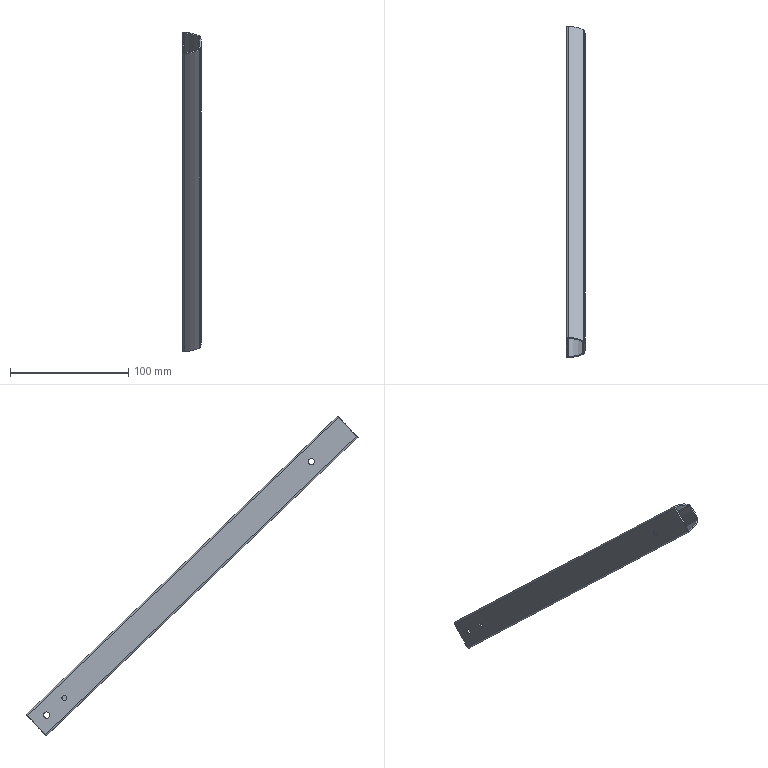Part | SolidWorks | features BaseBody 1 | 1 solid | 30 faces | box 16 x 280.261 x 269.738 mm | volume 29192 mm3 | cylinder 26 | plane 4 | commonest cylinder face diameters 5.2 x8 0.6 x3 3 x3 3.6 x2 4.2 x2 6 x2
STEP:
#1=CARTESIAN_POINT('',(173.2,660.373,82.941));
#2=VERTEX_POINT('',#1);
#3=CARTESIAN_POINT('',(173.2,660.373,87.141));
#4=VERTEX_POINT('',#3);
#5=CARTESIAN_POINT('',(173.2,660.373,85.041));
#6=DIRECTION('',(-1.,0.,0.));
#7=DIRECTION('',(0.,0.,1.));
#8=AXIS2_PLACEMENT_3D('',#5,#6,#7);
#9=CIRCLE('',#8,2.1);
#10=EDGE_CURVE('',#2,#4,#9,.T.);
#11=ORIENTED_EDGE('',*,*,#10,.F.);
#12=CARTESIAN_POINT('',(172.,660.373,82.941));
#13=VERTEX_POINT('',#12);
#14=CARTESIAN_POINT('',(182.,660.373,82.941));
#15=DIRECTION('',(-1.,0.,0.));
#16=VECTOR('',#15,1000.);
#17=LINE('',#14,#16);
#18=EDGE_CURVE('',#2,#13,#17,.T.);
#19=ORIENTED_EDGE('',*,*,#18,.T.);
#20=CARTESIAN_POINT('',(172.,660.373,87.141));
#21=VERTEX_POINT('',#20);
#22=CARTESIAN_POINT('',(172.,660.373,85.041));
#23=DIRECTION('',(1.,0.,0.));
#24=DIRECTION('',(0.,0.,1.));
#25=AXIS2_PLACEMENT_3D('',#22,#23,#24);
#26=CIRCLE('',#25,2.1);
#27=EDGE_CURVE('',#21,#13,#26,.T.);
#28=ORIENTED_EDGE('',*,*,#27,.F.);
#29=CARTESIAN_POINT('',(182.,660.373,87.141));
#30=DIRECTION('',(-1.,0.,0.));
#31=VECTOR('',#30,1000.);
#32=LINE('',#29,#31);
#33=EDGE_CURVE('',#4,#21,#32,.T.);
#34=ORIENTED_EDGE('',*,*,#33,.F.);
#35=EDGE_LOOP('',(#11,#19,#28,#34));
#36=FACE_OUTER_BOUND('',#35,.T.);
#37=CARTESIAN_POINT('',(182.,660.373,85.041));
#38=DIRECTION('',(-1.,0.,0.));
#39=DIRECTION('',(0.,0.,1.));
#40=AXIS2_PLACEMENT_3D('',#37,#38,#39);
#41=CYLINDRICAL_SURFACE('',#40,2.1);
#42=ADVANCED_FACE('',(#36),#41,.F.);
#43=CARTESIAN_POINT('',(172.,675.31,73.346));
#44=VERTEX_POINT('',#43);
#45=CARTESIAN_POINT('',(172.,675.31,68.146));
#46=VERTEX_POINT('',#45);
#47=CARTESIAN_POINT('',(172.,675.31,70.746));
#48=DIRECTION('',(1.,0.,0.));
#49=DIRECTION('',(0.,0.,-1.));
#50=AXIS2_PLACEMENT_3D('',#47,#48,#49);
#51=CIRCLE('',#50,2.6);
#52=EDGE_CURVE('',#44,#46,#51,.T.);
#53=ORIENTED_EDGE('',*,*,#52,.F.);
#54=CARTESIAN_POINT('',(173.2,675.31,73.346));
#55=VERTEX_POINT('',#54);
#56=CARTESIAN_POINT('',(133.,675.31,73.346));
#57=DIRECTION('',(1.,0.,0.));
#58=VECTOR('',#57,1000.);
#59=LINE('',#56,#58);
#60=EDGE_CURVE('',#44,#55,#59,.T.);
#61=ORIENTED_EDGE('',*,*,#60,.T.);
#62=CARTESIAN_POINT('',(173.2,675.31,68.146));
#63=VERTEX_POINT('',#62);
#64=CARTESIAN_POINT('',(173.2,675.31,70.746));
#65=DIRECTION('',(-1.,0.,0.));
#66=DIRECTION('',(0.,0.,-1.));
#67=AXIS2_PLACEMENT_3D('',#64,#65,#66);
#68=CIRCLE('',#67,2.6);
#69=EDGE_CURVE('',#63,#55,#68,.T.);
#70=ORIENTED_EDGE('',*,*,#69,.F.);
#71=CARTESIAN_POINT('',(133.,675.31,68.146));
#72=DIRECTION('',(1.,0.,0.));
#73=VECTOR('',#72,1000.);
#74=LINE('',#71,#73);
#75=EDGE_CURVE('',#46,#63,#74,.T.);
#76=ORIENTED_EDGE('',*,*,#75,.F.);
#77=EDGE_LOOP('',(#53,#61,#70,#76));
#78=FACE_OUTER_BOUND('',#77,.T.);
#79=CARTESIAN_POINT('',(133.,675.31,70.746));
#80=DIRECTION('',(1.,0.,0.));
#81=DIRECTION('',(0.,0.,-1.));
#82=AXIS2_PLACEMENT_3D('',#79,#80,#81);
#83=CYLINDRICAL_SURFACE('',#82,2.6);
#84=ADVANCED_FACE('',(#78),#83,.F.);
#85=CARTESIAN_POINT('',(172.,428.723,321.908));
#86=VERTEX_POINT('',#85);
#87=CARTESIAN_POINT('',(173.5,429.76,322.992));
#88=VERTEX_POINT('',#87);
#89=CARTESIAN_POINT('',(173.5,428.723,321.908));
#90=DIRECTION('',(0.,0.7224,-0.6914));
#91=DIRECTION('',(0.,0.6914,0.7224));
#92=AXIS2_PLACEMENT_3D('',#89,#90,#91);
#93=CIRCLE('',#92,1.5);
#94=EDGE_CURVE('',#86,#88,#93,.T.);
#95=ORIENTED_EDGE('',*,*,#94,.T.);
#96=CARTESIAN_POINT('',(173.5,692.797,71.25));
#97=VERTEX_POINT('',#96);
#98=CARTESIAN_POINT('',(173.5,-6.027,740.064));
#99=DIRECTION('',(0.,0.7224,-0.6914));
#100=VECTOR('',#99,1000.);
#101=LINE('',#98,#100);
#102=EDGE_CURVE('',#88,#97,#101,.T.);
#103=ORIENTED_EDGE('',*,*,#102,.T.);
#104=CARTESIAN_POINT('',(172.,691.76,70.167));
#105=VERTEX_POINT('',#104);
#106=CARTESIAN_POINT('',(173.5,691.76,70.167));
#107=DIRECTION('',(0.,0.7224,-0.6914));
#108=DIRECTION('',(0.,0.6914,0.7224));
#109=AXIS2_PLACEMENT_3D('',#106,#107,#108);
#110=CIRCLE('',#109,1.5);
#111=EDGE_CURVE('',#105,#97,#110,.T.);
#112=ORIENTED_EDGE('',*,*,#111,.F.);
#113=CARTESIAN_POINT('',(172.,428.723,321.908));
#114=DIRECTION('',(0.,0.7224,-0.6914));
#115=VECTOR('',#114,1000.);
#116=LINE('',#113,#115);
#117=EDGE_CURVE('',#86,#105,#116,.T.);
#118=ORIENTED_EDGE('',*,*,#117,.F.);
#119=EDGE_LOOP('',(#95,#103,#112,#118));
#120=FACE_OUTER_BOUND('',#119,.T.);
#121=CARTESIAN_POINT('',(173.5,-7.064,738.98));
#122=DIRECTION('',(0.,0.7224,-0.6914));
#123=DIRECTION('',(0.,0.6914,0.7224));
#124=AXIS2_PLACEMENT_3D('',#121,#122,#123);
#125=CYLINDRICAL_SURFACE('',#124,1.5);
#126=ADVANCED_FACE('',(#120),#125,.T.);
#127=CARTESIAN_POINT('',(172.,451.846,287.213));
#128=VERTEX_POINT('',#127);
#129=CARTESIAN_POINT('',(172.,451.846,282.013));
#130=VERTEX_POINT('',#129);
#131=CARTESIAN_POINT('',(172.,451.846,284.613));
#132=DIRECTION('',(1.,0.,0.));
#133=DIRECTION('',(0.,0.,-1.));
#134=AXIS2_PLACEMENT_3D('',#131,#132,#133);
#135=CIRCLE('',#134,2.6);
#136=EDGE_CURVE('',#128,#130,#135,.T.);
#137=ORIENTED_EDGE('',*,*,#136,.F.);
#138=CARTESIAN_POINT('',(173.2,451.846,287.213));
#139=VERTEX_POINT('',#138);
#140=CARTESIAN_POINT('',(-462.,451.846,287.213));
#141=DIRECTION('',(1.,0.,0.));
#142=VECTOR('',#141,1000.);
#143=LINE('',#140,#142);
#144=EDGE_CURVE('',#128,#139,#143,.T.);
#145=ORIENTED_EDGE('',*,*,#144,.T.);
#146=CARTESIAN_POINT('',(173.2,451.846,282.013));
#147=VERTEX_POINT('',#146);
#148=CARTESIAN_POINT('',(173.2,451.846,284.613));
#149=DIRECTION('',(-1.,0.,0.));
#150=DIRECTION('',(0.,0.,-1.));
#151=AXIS2_PLACEMENT_3D('',#148,#149,#150);
#152=CIRCLE('',#151,2.6);
#153=EDGE_CURVE('',#147,#139,#152,.T.);
#154=ORIENTED_EDGE('',*,*,#153,.F.);
#155=CARTESIAN_POINT('',(-462.,451.846,282.013));
#156=DIRECTION('',(1.,0.,0.));
#157=VECTOR('',#156,1000.);
#158=LINE('',#155,#157);
#159=EDGE_CURVE('',#130,#147,#158,.T.);
#160=ORIENTED_EDGE('',*,*,#159,.F.);
#161=EDGE_LOOP('',(#137,#145,#154,#160));
#162=FACE_OUTER_BOUND('',#161,.T.);
#163=CARTESIAN_POINT('',(-462.,451.846,284.613));
#164=DIRECTION('',(1.,0.,0.));
#165=DIRECTION('',(0.,0.,-1.));
#166=AXIS2_PLACEMENT_3D('',#163,#164,#165);
#167=CYLINDRICAL_SURFACE('',#166,2.6);
#168=ADVANCED_FACE('',(#162),#167,.F.);
#169=CARTESIAN_POINT('',(173.5,428.93,322.125));
#170=VERTEX_POINT('',#169);
#171=CARTESIAN_POINT('',(173.519,428.93,322.124));
#172=VERTEX_POINT('',#171);
#173=CARTESIAN_POINT('',(173.5,428.723,321.908));
#174=DIRECTION('',(0.,0.7224,-0.6914));
#175=DIRECTION('',(0.,0.6914,0.7224));
#176=AXIS2_PLACEMENT_3D('',#173,#174,#175);
#177=CIRCLE('',#176,0.3);
#178=EDGE_CURVE('',#170,#172,#177,.T.);
#179=ORIENTED_EDGE('',*,*,#178,.F.);
#180=CARTESIAN_POINT('',(173.5,691.967,70.383));
#181=VERTEX_POINT('',#180);
#182=CARTESIAN_POINT('',(173.5,-6.857,739.197));
#183=DIRECTION('',(0.,0.7224,-0.6914));
#184=VECTOR('',#183,1000.);
#185=LINE('',#182,#184);
#186=EDGE_CURVE('',#170,#181,#185,.T.);
#187=ORIENTED_EDGE('',*,*,#186,.T.);
#188=CARTESIAN_POINT('',(173.519,691.967,70.383));
#189=VERTEX_POINT('',#188);
#190=CARTESIAN_POINT('',(173.5,691.76,70.167));
#191=DIRECTION('',(0.,-0.7224,0.6914));
#192=DIRECTION('',(0.,0.6914,0.7224));
#193=AXIS2_PLACEMENT_3D('',#190,#191,#192);
#194=CIRCLE('',#193,0.3);
#195=EDGE_CURVE('',#189,#181,#194,.T.);
#196=ORIENTED_EDGE('',*,*,#195,.F.);
#197=CARTESIAN_POINT('',(173.519,-6.857,739.196));
#198=DIRECTION('',(0.,-0.7224,0.6914));
#199=VECTOR('',#198,1000.);
#200=LINE('',#197,#199);
#201=EDGE_CURVE('',#189,#172,#200,.T.);
#202=ORIENTED_EDGE('',*,*,#201,.T.);
#203=EDGE_LOOP('',(#179,#187,#196,#202));
#204=FACE_OUTER_BOUND('',#203,.T.);
#205=CARTESIAN_POINT('',(173.5,-7.064,738.98));
#206=DIRECTION('',(0.,0.7224,-0.6914));
#207=DIRECTION('',(0.,0.6914,0.7224));
#208=AXIS2_PLACEMENT_3D('',#205,#206,#207);
#209=CYLINDRICAL_SURFACE('',#208,0.3);
#210=ADVANCED_FACE('',(#204),#209,.F.);
#211=CARTESIAN_POINT('',(186.739,675.31,68.146));
#212=VERTEX_POINT('',#211);
#213=CARTESIAN_POINT('',(186.739,675.31,73.346));
#214=VERTEX_POINT('',#213);
#215=CARTESIAN_POINT('',(186.739,675.31,68.146));
#216=CARTESIAN_POINT('',(186.731,675.138,68.146));
#217=CARTESIAN_POINT('',(186.723,674.969,68.163));
#218=CARTESIAN_POINT('',(186.709,674.637,68.229));
#219=CARTESIAN_POINT('',(186.703,674.472,68.279));
#220=CARTESIAN_POINT('',(186.693,674.157,68.41));
#221=CARTESIAN_POINT('',(186.689,674.008,68.49));
#222=CARTESIAN_POINT('',(186.683,673.725,68.678));
#223=CARTESIAN_POINT('',(186.682,673.591,68.788));
#224=CARTESIAN_POINT('',(186.683,673.351,69.028));
#225=CARTESIAN_POINT('',(186.685,673.244,69.159));
#226=CARTESIAN_POINT('',(186.691,673.053,69.443));
#227=CARTESIAN_POINT('',(186.696,672.973,69.595));
#228=CARTESIAN_POINT('',(186.707,672.843,69.907));
#229=CARTESIAN_POINT('',(186.714,672.793,70.071));
#230=CARTESIAN_POINT('',(186.728,672.726,70.407));
#231=CARTESIAN_POINT('',(186.736,672.71,70.575));
#232=CARTESIAN_POINT('',(186.751,672.71,70.914));
#233=CARTESIAN_POINT('',(186.759,672.726,71.086));
#234=CARTESIAN_POINT('',(186.773,672.793,71.42));
#235=CARTESIAN_POINT('',(186.779,672.842,71.582));
#236=CARTESIAN_POINT('',(186.79,672.972,71.896));
#237=CARTESIAN_POINT('',(186.794,673.053,72.049));
#238=CARTESIAN_POINT('',(186.799,673.241,72.331));
#239=CARTESIAN_POINT('',(186.8,673.349,72.462));
#240=CARTESIAN_POINT('',(186.8,673.591,72.705));
#241=CARTESIAN_POINT('',(186.798,673.723,72.813));
#242=CARTESIAN_POINT('',(186.791,674.004,73.001));
#243=CARTESIAN_POINT('',(186.787,674.156,73.083));
#244=CARTESIAN_POINT('',(186.775,674.471,73.213));
#245=CARTESIAN_POINT('',(186.769,674.633,73.263));
#246=CARTESIAN_POINT('',(186.754,674.966,73.329));
#247=CARTESIAN_POINT('',(186.746,675.138,73.346));
#248=CARTESIAN_POINT('',(186.739,675.31,73.346));
#249=B_SPLINE_CURVE_WITH_KNOTS('',3,(#215,#216,#217,#218,#219,#220,#221,#222,#223,#224,#225,#226,#227,#228,#229,#230,#231,#232,#233,#234,#235,#236,#237,#238,#239,#240,#241,#242,#243,#244,#245,#246,#247,#248),.UNSPECIFIED.,.F.,.F.,(4,2,2,2,2,2,2,2,2,2,2,2,2,2,2,2,4),(0.,0.0005082,0.001016,0.001525,0.002033,0.002541,0.003049,0.003557,0.004066,0.004574,0.005082,0.00559,0.006098,0.006607,0.007115,0.007623,0.008131),.UNSPECIFIED.);
#250=EDGE_CURVE('',#212,#214,#249,.T.);
#251=ORIENTED_EDGE('',*,*,#250,.T.);
#252=CARTESIAN_POINT('',(187.941,675.31,73.346));
#253=VERTEX_POINT('',#252);
#254=CARTESIAN_POINT('',(133.,675.31,73.346));
#255=DIRECTION('',(1.,0.,0.));
#256=VECTOR('',#255,1000.);
#257=LINE('',#254,#256);
#258=EDGE_CURVE('',#214,#253,#257,.T.);
#259=ORIENTED_EDGE('',*,*,#258,.T.);
#260=CARTESIAN_POINT('',(187.941,675.31,68.146));
#261=VERTEX_POINT('',#260);
#262=CARTESIAN_POINT('',(187.941,675.31,68.146));
#263=CARTESIAN_POINT('',(187.934,675.138,68.146));
#264=CARTESIAN_POINT('',(187.926,674.969,68.163));
#265=CARTESIAN_POINT('',(187.913,674.637,68.229));
#266=CARTESIAN_POINT('',(187.907,674.472,68.279));
#267=CARTESIAN_POINT('',(187.897,674.157,68.41));
#268=CARTESIAN_POINT('',(187.893,674.008,68.49));
#269=CARTESIAN_POINT('',(187.888,673.725,68.678));
#270=CARTESIAN_POINT('',(187.887,673.591,68.788));
#271=CARTESIAN_POINT('',(187.887,673.351,69.028));
#272=CARTESIAN_POINT('',(187.889,673.244,69.159));
#273=CARTESIAN_POINT('',(187.896,673.053,69.443));
#274=CARTESIAN_POINT('',(187.9,672.973,69.595));
#275=CARTESIAN_POINT('',(187.911,672.843,69.907));
#276=CARTESIAN_POINT('',(187.917,672.793,70.071));
#277=CARTESIAN_POINT('',(187.931,672.726,70.407));
#278=CARTESIAN_POINT('',(187.939,672.71,70.575));
#279=CARTESIAN_POINT('',(187.953,672.71,70.914));
#280=CARTESIAN_POINT('',(187.961,672.726,71.086));
#281=CARTESIAN_POINT('',(187.974,672.793,71.42));
#282=CARTESIAN_POINT('',(187.98,672.842,71.582));
#283=CARTESIAN_POINT('',(187.99,672.972,71.896));
#284=CARTESIAN_POINT('',(187.994,673.053,72.049));
#285=CARTESIAN_POINT('',(187.999,673.241,72.331));
#286=CARTESIAN_POINT('',(188.,673.349,72.462));
#287=CARTESIAN_POINT('',(188.,673.591,72.705));
#288=CARTESIAN_POINT('',(187.998,673.723,72.813));
#289=CARTESIAN_POINT('',(187.992,674.004,73.001));
#290=CARTESIAN_POINT('',(187.987,674.156,73.083));
#291=CARTESIAN_POINT('',(187.976,674.471,73.213));
#292=CARTESIAN_POINT('',(187.97,674.633,73.263));
#293=CARTESIAN_POINT('',(187.956,674.966,73.329));
#294=CARTESIAN_POINT('',(187.949,675.138,73.346));
#295=CARTESIAN_POINT('',(187.941,675.31,73.346));
#296=B_SPLINE_CURVE_WITH_KNOTS('',3,(#262,#263,#264,#265,#266,#267,#268,#269,#270,#271,#272,#273,#274,#275,#276,#277,#278,#279,#280,#281,#282,#283,#284,#285,#286,#287,#288,#289,#290,#291,#292,#293,#294,#295),.UNSPECIFIED.,.F.,.F.,(4,2,2,2,2,2,2,2,2,2,2,2,2,2,2,2,4),(0.008131,0.008639,0.009147,0.009655,0.01016,0.01067,0.01118,0.01169,0.0122,0.0127,0.01321,0.01372,0.01423,0.01474,0.01525,0.01575,0.01626),.UNSPECIFIED.);
#297=EDGE_CURVE('',#261,#253,#296,.T.);
#298=ORIENTED_EDGE('',*,*,#297,.F.);
#299=CARTESIAN_POINT('',(133.,675.31,68.146));
#300=DIRECTION('',(1.,0.,0.));
#301=VECTOR('',#300,1000.);
#302=LINE('',#299,#301);
#303=EDGE_CURVE('',#212,#261,#302,.T.);
#304=ORIENTED_EDGE('',*,*,#303,.F.);
#305=EDGE_LOOP('',(#251,#259,#298,#304));
#306=FACE_OUTER_BOUND('',#305,.T.);
#307=CARTESIAN_POINT('',(133.,675.31,70.746));
#308=DIRECTION('',(1.,0.,0.));
#309=DIRECTION('',(0.,0.,-1.));
#310=AXIS2_PLACEMENT_3D('',#307,#308,#309);
#311=CYLINDRICAL_SURFACE('',#310,2.6);
#312=ADVANCED_FACE('',(#306),#311,.F.);
#313=CARTESIAN_POINT('',(186.739,451.846,282.013));
#314=VERTEX_POINT('',#313);
#315=CARTESIAN_POINT('',(186.739,451.846,287.213));
#316=VERTEX_POINT('',#315);
#317=CARTESIAN_POINT('',(186.739,451.846,282.013));
#318=CARTESIAN_POINT('',(186.731,451.675,282.013));
#319=CARTESIAN_POINT('',(186.723,451.506,282.03));
#320=CARTESIAN_POINT('',(186.709,451.174,282.096));
#321=CARTESIAN_POINT('',(186.703,451.009,282.146));
#322=CARTESIAN_POINT('',(186.693,450.694,282.276));
#323=CARTESIAN_POINT('',(186.689,450.545,282.356));
#324=CARTESIAN_POINT('',(186.683,450.262,282.545));
#325=CARTESIAN_POINT('',(186.682,450.128,282.655));
#326=CARTESIAN_POINT('',(186.683,449.888,282.895));
#327=CARTESIAN_POINT('',(186.685,449.78,283.026));
#328=CARTESIAN_POINT('',(186.691,449.59,283.31));
#329=CARTESIAN_POINT('',(186.696,449.509,283.461));
#330=CARTESIAN_POINT('',(186.707,449.38,283.774));
#331=CARTESIAN_POINT('',(186.714,449.33,283.938));
#332=CARTESIAN_POINT('',(186.728,449.263,284.273));
#333=CARTESIAN_POINT('',(186.736,449.247,284.442));
#334=CARTESIAN_POINT('',(186.751,449.246,284.781));
#335=CARTESIAN_POINT('',(186.759,449.263,284.953));
#336=CARTESIAN_POINT('',(186.773,449.329,285.286));
#337=CARTESIAN_POINT('',(186.779,449.378,285.448));
#338=CARTESIAN_POINT('',(186.79,449.508,285.763));
#339=CARTESIAN_POINT('',(186.794,449.59,285.915));
#340=CARTESIAN_POINT('',(186.799,449.778,286.197));
#341=CARTESIAN_POINT('',(186.8,449.885,286.329));
#342=CARTESIAN_POINT('',(186.8,450.128,286.572));
#343=CARTESIAN_POINT('',(186.798,450.26,286.68));
#344=CARTESIAN_POINT('',(186.791,450.541,286.868));
#345=CARTESIAN_POINT('',(186.787,450.693,286.95));
#346=CARTESIAN_POINT('',(186.775,451.008,287.08));
#347=CARTESIAN_POINT('',(186.769,451.17,287.129));
#348=CARTESIAN_POINT('',(186.754,451.503,287.196));
#349=CARTESIAN_POINT('',(186.746,451.675,287.213));
#350=CARTESIAN_POINT('',(186.739,451.846,287.213));
#351=B_SPLINE_CURVE_WITH_KNOTS('',3,(#317,#318,#319,#320,#321,#322,#323,#324,#325,#326,#327,#328,#329,#330,#331,#332,#333,#334,#335,#336,#337,#338,#339,#340,#341,#342,#343,#344,#345,#346,#347,#348,#349,#350),.UNSPECIFIED.,.F.,.F.,(4,2,2,2,2,2,2,2,2,2,2,2,2,2,2,2,4),(0.,0.0005082,0.001016,0.001525,0.002033,0.002541,0.003049,0.003557,0.004066,0.004574,0.005082,0.00559,0.006098,0.006607,0.007115,0.007623,0.008131),.UNSPECIFIED.);
#352=EDGE_CURVE('',#314,#316,#351,.T.);
#353=ORIENTED_EDGE('',*,*,#352,.T.);
#354=CARTESIAN_POINT('',(187.941,451.846,287.213));
#355=VERTEX_POINT('',#354);
#356=CARTESIAN_POINT('',(-462.,451.846,287.213));
#357=DIRECTION('',(1.,0.,0.));
#358=VECTOR('',#357,1000.);
#359=LINE('',#356,#358);
#360=EDGE_CURVE('',#316,#355,#359,.T.);
#361=ORIENTED_EDGE('',*,*,#360,.T.);
#362=CARTESIAN_POINT('',(187.941,451.846,282.013));
#363=VERTEX_POINT('',#362);
#364=CARTESIAN_POINT('',(187.941,451.846,282.013));
#365=CARTESIAN_POINT('',(187.934,451.675,282.013));
#366=CARTESIAN_POINT('',(187.926,451.506,282.03));
#367=CARTESIAN_POINT('',(187.913,451.174,282.096));
#368=CARTESIAN_POINT('',(187.907,451.009,282.146));
#369=CARTESIAN_POINT('',(187.897,450.694,282.276));
#370=CARTESIAN_POINT('',(187.893,450.545,282.356));
#371=CARTESIAN_POINT('',(187.888,450.262,282.545));
#372=CARTESIAN_POINT('',(187.887,450.128,282.655));
#373=CARTESIAN_POINT('',(187.887,449.888,282.895));
#374=CARTESIAN_POINT('',(187.889,449.78,283.026));
#375=CARTESIAN_POINT('',(187.896,449.59,283.31));
#376=CARTESIAN_POINT('',(187.9,449.509,283.461));
#377=CARTESIAN_POINT('',(187.911,449.38,283.774));
#378=CARTESIAN_POINT('',(187.917,449.33,283.938));
#379=CARTESIAN_POINT('',(187.931,449.263,284.273));
#380=CARTESIAN_POINT('',(187.939,449.247,284.442));
#381=CARTESIAN_POINT('',(187.953,449.246,284.781));
#382=CARTESIAN_POINT('',(187.961,449.263,284.953));
#383=CARTESIAN_POINT('',(187.974,449.329,285.286));
#384=CARTESIAN_POINT('',(187.98,449.378,285.448));
#385=CARTESIAN_POINT('',(187.99,449.508,285.763));
#386=CARTESIAN_POINT('',(187.994,449.59,285.915));
#387=CARTESIAN_POINT('',(187.999,449.778,286.197));
#388=CARTESIAN_POINT('',(188.,449.885,286.329));
#389=CARTESIAN_POINT('',(188.,450.128,286.572));
#390=CARTESIAN_POINT('',(187.998,450.26,286.68));
#391=CARTESIAN_POINT('',(187.992,450.541,286.868));
#392=CARTESIAN_POINT('',(187.987,450.693,286.95));
#393=CARTESIAN_POINT('',(187.976,451.008,287.08));
#394=CARTESIAN_POINT('',(187.97,451.17,287.129));
#395=CARTESIAN_POINT('',(187.956,451.503,287.196));
#396=CARTESIAN_POINT('',(187.949,451.675,287.213));
#397=CARTESIAN_POINT('',(187.941,451.846,287.213));
#398=B_SPLINE_CURVE_WITH_KNOTS('',3,(#364,#365,#366,#367,#368,#369,#370,#371,#372,#373,#374,#375,#376,#377,#378,#379,#380,#381,#382,#383,#384,#385,#386,#387,#388,#389,#390,#391,#392,#393,#394,#395,#396,#397),.UNSPECIFIED.,.F.,.F.,(4,2,2,2,2,2,2,2,2,2,2,2,2,2,2,2,4),(0.008131,0.008639,0.009147,0.009655,0.01016,0.01067,0.01118,0.01169,0.0122,0.0127,0.01321,0.01372,0.01423,0.01474,0.01525,0.01575,0.01626),.UNSPECIFIED.);
#399=EDGE_CURVE('',#363,#355,#398,.T.);
#400=ORIENTED_EDGE('',*,*,#399,.F.);
#401=CARTESIAN_POINT('',(-462.,451.846,282.013));
#402=DIRECTION('',(1.,0.,0.));
#403=VECTOR('',#402,1000.);
#404=LINE('',#401,#403);
#405=EDGE_CURVE('',#314,#363,#404,.T.);
#406=ORIENTED_EDGE('',*,*,#405,.F.);
#407=EDGE_LOOP('',(#353,#361,#400,#406));
#408=FACE_OUTER_BOUND('',#407,.T.);
#409=CARTESIAN_POINT('',(-462.,451.846,284.613));
#410=DIRECTION('',(1.,0.,0.));
#411=DIRECTION('',(0.,0.,-1.));
#412=AXIS2_PLACEMENT_3D('',#409,#410,#411);
#413=CYLINDRICAL_SURFACE('',#412,2.6);
#414=ADVANCED_FACE('',(#408),#413,.F.);
#415=ORIENTED_EDGE('',*,*,#27,.T.);
#416=CARTESIAN_POINT('',(172.,660.373,85.041));
#417=DIRECTION('',(1.,0.,0.));
#418=DIRECTION('',(0.,0.,1.));
#419=AXIS2_PLACEMENT_3D('',#416,#417,#418);
#420=CIRCLE('',#419,2.1);
#421=EDGE_CURVE('',#13,#21,#420,.T.);
#422=ORIENTED_EDGE('',*,*,#421,.T.);
#423=EDGE_LOOP('',(#415,#422));
#424=FACE_BOUND('',#423,.T.);
#425=CARTESIAN_POINT('',(172.,675.31,70.746));
#426=DIRECTION('',(1.,0.,0.));
#427=DIRECTION('',(0.,0.,-1.));
#428=AXIS2_PLACEMENT_3D('',#425,#426,#427);
#429=CIRCLE('',#428,2.6);
#430=EDGE_CURVE('',#46,#44,#429,.T.);
#431=ORIENTED_EDGE('',*,*,#430,.T.);
#432=ORIENTED_EDGE('',*,*,#52,.T.);
#433=EDGE_LOOP('',(#431,#432));
#434=FACE_BOUND('',#433,.T.);
#435=CARTESIAN_POINT('',(172.,676.611,54.338));
#436=VERTEX_POINT('',#435);
#437=CARTESIAN_POINT('',(172.,691.76,70.167));
#438=DIRECTION('',(0.,-0.6914,-0.7224));
#439=VECTOR('',#438,1000.);
#440=LINE('',#437,#439);
#441=EDGE_CURVE('',#105,#436,#440,.T.);
#442=ORIENTED_EDGE('',*,*,#441,.T.);
#443=CARTESIAN_POINT('',(172.,413.573,306.079));
#444=VERTEX_POINT('',#443);
#445=CARTESIAN_POINT('',(172.,676.611,54.338));
#446=DIRECTION('',(0.,-0.7224,0.6914));
#447=VECTOR('',#446,1000.);
#448=LINE('',#445,#447);
#449=EDGE_CURVE('',#436,#444,#448,.T.);
#450=ORIENTED_EDGE('',*,*,#449,.T.);
#451=CARTESIAN_POINT('',(172.,413.573,306.079));
#452=DIRECTION('',(0.,0.6914,0.7224));
#453=VECTOR('',#452,1000.);
#454=LINE('',#451,#453);
#455=EDGE_CURVE('',#444,#86,#454,.T.);
#456=ORIENTED_EDGE('',*,*,#455,.T.);
#457=ORIENTED_EDGE('',*,*,#117,.T.);
#458=EDGE_LOOP('',(#442,#450,#456,#457));
#459=FACE_OUTER_BOUND('',#458,.T.);
#460=CARTESIAN_POINT('',(172.,451.846,284.613));
#461=DIRECTION('',(1.,0.,0.));
#462=DIRECTION('',(0.,0.,-1.));
#463=AXIS2_PLACEMENT_3D('',#460,#461,#462);
#464=CIRCLE('',#463,2.6);
#465=EDGE_CURVE('',#130,#128,#464,.T.);
#466=ORIENTED_EDGE('',*,*,#465,.T.);
#467=ORIENTED_EDGE('',*,*,#136,.T.);
#468=EDGE_LOOP('',(#466,#467));
#469=FACE_BOUND('',#468,.T.);
#470=CARTESIAN_POINT('',(172.,-22.214,723.151));
#471=DIRECTION('',(-1.,0.,0.));
#472=DIRECTION('',(0.,0.,1.));
#473=AXIS2_PLACEMENT_3D('',#470,#471,#472);
#474=PLANE('',#473);
#475=ADVANCED_FACE('',(#424,#434,#459,#469),#474,.T.);
#476=ORIENTED_EDGE('',*,*,#18,.F.);
#477=CARTESIAN_POINT('',(173.2,660.373,85.041));
#478=DIRECTION('',(-1.,0.,0.));
#479=DIRECTION('',(0.,0.,1.));
#480=AXIS2_PLACEMENT_3D('',#477,#478,#479);
#481=CIRCLE('',#480,2.1);
#482=EDGE_CURVE('',#4,#2,#481,.T.);
#483=ORIENTED_EDGE('',*,*,#482,.F.);
#484=ORIENTED_EDGE('',*,*,#33,.T.);
#485=ORIENTED_EDGE('',*,*,#421,.F.);
#486=EDGE_LOOP('',(#476,#483,#484,#485));
#487=FACE_OUTER_BOUND('',#486,.T.);
#488=CARTESIAN_POINT('',(182.,660.373,85.041));
#489=DIRECTION('',(-1.,0.,0.));
#490=DIRECTION('',(0.,0.,1.));
#491=AXIS2_PLACEMENT_3D('',#488,#489,#490);
#492=CYLINDRICAL_SURFACE('',#491,2.1);
#493=ADVANCED_FACE('',(#487),#492,.F.);
#494=ORIENTED_EDGE('',*,*,#60,.F.);
#495=ORIENTED_EDGE('',*,*,#430,.F.);
#496=ORIENTED_EDGE('',*,*,#75,.T.);
#497=CARTESIAN_POINT('',(173.2,675.31,70.746));
#498=DIRECTION('',(-1.,0.,0.));
#499=DIRECTION('',(0.,0.,-1.));
#500=AXIS2_PLACEMENT_3D('',#497,#498,#499);
#501=CIRCLE('',#500,2.6);
#502=EDGE_CURVE('',#55,#63,#501,.T.);
#503=ORIENTED_EDGE('',*,*,#502,.F.);
#504=EDGE_LOOP('',(#494,#495,#496,#503));
#505=FACE_OUTER_BOUND('',#504,.T.);
#506=CARTESIAN_POINT('',(133.,675.31,70.746));
#507=DIRECTION('',(1.,0.,0.));
#508=DIRECTION('',(0.,0.,-1.));
#509=AXIS2_PLACEMENT_3D('',#506,#507,#508);
#510=CYLINDRICAL_SURFACE('',#509,2.6);
#511=ADVANCED_FACE('',(#505),#510,.F.);
#512=CARTESIAN_POINT('',(173.593,675.576,53.256));
#513=VERTEX_POINT('',#512);
#514=CARTESIAN_POINT('',(173.5,676.611,54.338));
#515=DIRECTION('',(0.,-0.7224,0.6914));
#516=DIRECTION('',(0.,0.6914,0.7224));
#517=AXIS2_PLACEMENT_3D('',#514,#515,#516);
#518=CIRCLE('',#517,1.5);
#519=EDGE_CURVE('',#436,#513,#518,.T.);
#520=ORIENTED_EDGE('',*,*,#519,.T.);
#521=CARTESIAN_POINT('',(173.593,412.538,304.997));
#522=VERTEX_POINT('',#521);
#523=CARTESIAN_POINT('',(173.593,-23.249,722.069));
#524=DIRECTION('',(0.,-0.7224,0.6914));
#525=VECTOR('',#524,1000.);
#526=LINE('',#523,#525);
#527=EDGE_CURVE('',#513,#522,#526,.T.);
#528=ORIENTED_EDGE('',*,*,#527,.T.);
#529=CARTESIAN_POINT('',(173.5,413.573,306.079));
#530=DIRECTION('',(0.,0.7224,-0.6914));
#531=DIRECTION('',(0.,0.6914,0.7224));
#532=AXIS2_PLACEMENT_3D('',#529,#530,#531);
#533=CIRCLE('',#532,1.5);
#534=EDGE_CURVE('',#522,#444,#533,.T.);
#535=ORIENTED_EDGE('',*,*,#534,.T.);
#536=ORIENTED_EDGE('',*,*,#449,.F.);
#537=EDGE_LOOP('',(#520,#528,#535,#536));
#538=FACE_OUTER_BOUND('',#537,.T.);
#539=CARTESIAN_POINT('',(173.5,-22.214,723.151));
#540=DIRECTION('',(0.,0.7224,-0.6914));
#541=DIRECTION('',(0.,0.6914,0.7224));
#542=AXIS2_PLACEMENT_3D('',#539,#540,#541);
#543=CYLINDRICAL_SURFACE('',#542,1.5);
#544=ADVANCED_FACE('',(#538),#543,.T.);
#545=CARTESIAN_POINT('',(173.593,692.795,71.248));
#546=VERTEX_POINT('',#545);
#547=CARTESIAN_POINT('',(186.072,689.852,68.173));
#548=VERTEX_POINT('',#547);
#549=CARTESIAN_POINT('',(172.047,675.543,53.222));
#550=DIRECTION('',(0.,0.7224,-0.6914));
#551=DIRECTION('',(0.,0.6914,0.7224));
#552=AXIS2_PLACEMENT_3D('',#549,#550,#551);
#553=CIRCLE('',#552,25.);
#554=EDGE_CURVE('',#546,#548,#553,.T.);
#555=ORIENTED_EDGE('',*,*,#554,.T.);
#556=CARTESIAN_POINT('',(187.321,688.574,66.838));
#557=VERTEX_POINT('',#556);
#558=CARTESIAN_POINT('',(184.389,688.135,66.379));
#559=DIRECTION('',(0.,0.7224,-0.6914));
#560=DIRECTION('',(0.,0.6914,0.7224));
#561=AXIS2_PLACEMENT_3D('',#558,#559,#560);
#562=CIRCLE('',#561,3.);
#563=EDGE_CURVE('',#548,#557,#562,.T.);
#564=ORIENTED_EDGE('',*,*,#563,.T.);
#565=CARTESIAN_POINT('',(187.321,679.797,57.667));
#566=VERTEX_POINT('',#565);
#567=CARTESIAN_POINT('',(158.,684.185,62.252));
#568=DIRECTION('',(0.,0.7224,-0.6914));
#569=DIRECTION('',(0.,0.6914,0.7224));
#570=AXIS2_PLACEMENT_3D('',#567,#568,#569);
#571=CIRCLE('',#570,30.);
#572=EDGE_CURVE('',#557,#566,#571,.T.);
#573=ORIENTED_EDGE('',*,*,#572,.T.);
#574=CARTESIAN_POINT('',(186.072,678.518,56.331));
#575=VERTEX_POINT('',#574);
#576=CARTESIAN_POINT('',(184.389,680.236,58.125));
#577=DIRECTION('',(0.,0.7224,-0.6914));
#578=DIRECTION('',(0.,0.6914,0.7224));
#579=AXIS2_PLACEMENT_3D('',#576,#577,#578);
#580=CIRCLE('',#579,3.);
#581=EDGE_CURVE('',#566,#575,#580,.T.);
#582=ORIENTED_EDGE('',*,*,#581,.T.);
#583=CARTESIAN_POINT('',(172.047,692.828,71.283));
#584=DIRECTION('',(0.,0.7224,-0.6914));
#585=DIRECTION('',(0.,0.6914,0.7224));
#586=AXIS2_PLACEMENT_3D('',#583,#584,#585);
#587=CIRCLE('',#586,25.);
#588=EDGE_CURVE('',#575,#513,#587,.T.);
#589=ORIENTED_EDGE('',*,*,#588,.T.);
#590=ORIENTED_EDGE('',*,*,#519,.F.);
#591=ORIENTED_EDGE('',*,*,#441,.F.);
#592=ORIENTED_EDGE('',*,*,#111,.T.);
#593=CARTESIAN_POINT('',(173.5,691.76,70.167));
#594=DIRECTION('',(0.,0.7224,-0.6914));
#595=DIRECTION('',(0.,0.6914,0.7224));
#596=AXIS2_PLACEMENT_3D('',#593,#594,#595);
#597=CIRCLE('',#596,1.5);
#598=EDGE_CURVE('',#97,#546,#597,.T.);
#599=ORIENTED_EDGE('',*,*,#598,.T.);
#600=EDGE_LOOP('',(#555,#564,#573,#582,#589,#590,#591,#592,#599));
#601=FACE_OUTER_BOUND('',#600,.T.);
#602=CARTESIAN_POINT('',(186.148,688.398,66.654));
#603=VERTEX_POINT('',#602);
#604=CARTESIAN_POINT('',(185.399,689.165,67.456));
#605=VERTEX_POINT('',#604);
#606=CARTESIAN_POINT('',(184.389,688.135,66.379));
#607=DIRECTION('',(0.,-0.7224,0.6914));
#608=DIRECTION('',(0.,0.6914,0.7224));
#609=AXIS2_PLACEMENT_3D('',#606,#607,#608);
#610=CIRCLE('',#609,1.8);
#611=EDGE_CURVE('',#603,#605,#610,.T.);
#612=ORIENTED_EDGE('',*,*,#611,.T.);
#613=CARTESIAN_POINT('',(172.047,675.543,53.222));
#614=DIRECTION('',(0.,-0.7224,0.6914));
#615=DIRECTION('',(0.,0.6914,0.7224));
#616=AXIS2_PLACEMENT_3D('',#613,#614,#615);
#617=CIRCLE('',#616,23.8);
#618=EDGE_CURVE('',#605,#189,#617,.T.);
#619=ORIENTED_EDGE('',*,*,#618,.T.);
#620=ORIENTED_EDGE('',*,*,#195,.T.);
#621=CARTESIAN_POINT('',(173.2,691.76,70.167));
#622=VERTEX_POINT('',#621);
#623=CARTESIAN_POINT('',(173.5,691.76,70.167));
#624=DIRECTION('',(0.,-0.7224,0.6914));
#625=DIRECTION('',(0.,0.6914,0.7224));
#626=AXIS2_PLACEMENT_3D('',#623,#624,#625);
#627=CIRCLE('',#626,0.3);
#628=EDGE_CURVE('',#181,#622,#627,.T.);
#629=ORIENTED_EDGE('',*,*,#628,.T.);
#630=CARTESIAN_POINT('',(173.2,676.611,54.338));
#631=VERTEX_POINT('',#630);
#632=CARTESIAN_POINT('',(173.2,702.5,81.389));
#633=DIRECTION('',(0.,-0.6914,-0.7224));
#634=VECTOR('',#633,1000.);
#635=LINE('',#632,#634);
#636=EDGE_CURVE('',#622,#631,#635,.T.);
#637=ORIENTED_EDGE('',*,*,#636,.T.);
#638=CARTESIAN_POINT('',(173.519,676.404,54.121));
#639=VERTEX_POINT('',#638);
#640=CARTESIAN_POINT('',(173.5,676.611,54.338));
#641=DIRECTION('',(0.,-0.7224,0.6914));
#642=DIRECTION('',(0.,0.6914,0.7224));
#643=AXIS2_PLACEMENT_3D('',#640,#641,#642);
#644=CIRCLE('',#643,0.3);
#645=EDGE_CURVE('',#631,#639,#644,.T.);
#646=ORIENTED_EDGE('',*,*,#645,.T.);
#647=CARTESIAN_POINT('',(185.399,679.205,57.049));
#648=VERTEX_POINT('',#647);
#649=CARTESIAN_POINT('',(172.047,692.828,71.283));
#650=DIRECTION('',(0.,-0.7224,0.6914));
#651=DIRECTION('',(0.,0.6914,0.7224));
#652=AXIS2_PLACEMENT_3D('',#649,#650,#651);
#653=CIRCLE('',#652,23.8);
#654=EDGE_CURVE('',#639,#648,#653,.T.);
#655=ORIENTED_EDGE('',*,*,#654,.T.);
#656=CARTESIAN_POINT('',(186.148,679.972,57.85));
#657=VERTEX_POINT('',#656);
#658=CARTESIAN_POINT('',(184.389,680.236,58.125));
#659=DIRECTION('',(0.,-0.7224,0.6914));
#660=DIRECTION('',(0.,0.6914,0.7224));
#661=AXIS2_PLACEMENT_3D('',#658,#659,#660);
#662=CIRCLE('',#661,1.8);
#663=EDGE_CURVE('',#648,#657,#662,.T.);
#664=ORIENTED_EDGE('',*,*,#663,.T.);
#665=CARTESIAN_POINT('',(158.,684.185,62.252));
#666=DIRECTION('',(0.,-0.7224,0.6914));
#667=DIRECTION('',(0.,0.6914,0.7224));
#668=AXIS2_PLACEMENT_3D('',#665,#666,#667);
#669=CIRCLE('',#668,28.8);
#670=EDGE_CURVE('',#657,#603,#669,.T.);
#671=ORIENTED_EDGE('',*,*,#670,.T.);
#672=EDGE_LOOP('',(#612,#619,#620,#629,#637,#646,#655,#664,#671));
#673=FACE_BOUND('',#672,.T.);
#674=CARTESIAN_POINT('',(188.821,702.5,81.389));
#675=DIRECTION('',(0.,0.7224,-0.6914));
#676=DIRECTION('',(0.,0.6914,0.7224));
#677=AXIS2_PLACEMENT_3D('',#674,#675,#676);
#678=PLANE('',#677);
#679=ADVANCED_FACE('',(#601,#673),#678,.T.);
#680=ORIENTED_EDGE('',*,*,#102,.F.);
#681=CARTESIAN_POINT('',(173.593,429.758,322.99));
#682=VERTEX_POINT('',#681);
#683=CARTESIAN_POINT('',(173.5,428.723,321.908));
#684=DIRECTION('',(0.,0.7224,-0.6914));
#685=DIRECTION('',(0.,0.6914,0.7224));
#686=AXIS2_PLACEMENT_3D('',#683,#684,#685);
#687=CIRCLE('',#686,1.5);
#688=EDGE_CURVE('',#88,#682,#687,.T.);
#689=ORIENTED_EDGE('',*,*,#688,.T.);
#690=CARTESIAN_POINT('',(173.593,-6.029,740.062));
#691=DIRECTION('',(0.,-0.7224,0.6914));
#692=VECTOR('',#691,1000.);
#693=LINE('',#690,#692);
#694=EDGE_CURVE('',#546,#682,#693,.T.);
#695=ORIENTED_EDGE('',*,*,#694,.F.);
#696=ORIENTED_EDGE('',*,*,#598,.F.);
#697=EDGE_LOOP('',(#680,#689,#695,#696));
#698=FACE_OUTER_BOUND('',#697,.T.);
#699=CARTESIAN_POINT('',(173.5,-7.064,738.98));
#700=DIRECTION('',(0.,0.7224,-0.6914));
#701=DIRECTION('',(0.,0.6914,0.7224));
#702=AXIS2_PLACEMENT_3D('',#699,#700,#701);
#703=CYLINDRICAL_SURFACE('',#702,1.5);
#704=ADVANCED_FACE('',(#698),#703,.T.);
#705=CARTESIAN_POINT('',(186.072,415.481,308.072));
#706=VERTEX_POINT('',#705);
#707=CARTESIAN_POINT('',(172.047,429.791,323.024));
#708=DIRECTION('',(0.,0.7224,-0.6914));
#709=DIRECTION('',(0.,0.6914,0.7224));
#710=AXIS2_PLACEMENT_3D('',#707,#708,#709);
#711=CIRCLE('',#710,25.);
#712=EDGE_CURVE('',#706,#522,#711,.T.);
#713=ORIENTED_EDGE('',*,*,#712,.F.);
#714=CARTESIAN_POINT('',(187.321,416.759,309.408));
#715=VERTEX_POINT('',#714);
#716=CARTESIAN_POINT('',(184.389,417.198,309.867));
#717=DIRECTION('',(0.,0.7224,-0.6914));
#718=DIRECTION('',(0.,0.6914,0.7224));
#719=AXIS2_PLACEMENT_3D('',#716,#717,#718);
#720=CIRCLE('',#719,3.);
#721=EDGE_CURVE('',#715,#706,#720,.T.);
#722=ORIENTED_EDGE('',*,*,#721,.F.);
#723=CARTESIAN_POINT('',(187.321,425.536,318.579));
#724=VERTEX_POINT('',#723);
#725=CARTESIAN_POINT('',(158.,421.148,313.993));
#726=DIRECTION('',(0.,0.7224,-0.6914));
#727=DIRECTION('',(0.,0.6914,0.7224));
#728=AXIS2_PLACEMENT_3D('',#725,#726,#727);
#729=CIRCLE('',#728,30.);
#730=EDGE_CURVE('',#724,#715,#729,.T.);
#731=ORIENTED_EDGE('',*,*,#730,.F.);
#732=CARTESIAN_POINT('',(186.072,426.815,319.915));
#733=VERTEX_POINT('',#732);
#734=CARTESIAN_POINT('',(184.389,425.098,318.12));
#735=DIRECTION('',(0.,0.7224,-0.6914));
#736=DIRECTION('',(0.,0.6914,0.7224));
#737=AXIS2_PLACEMENT_3D('',#734,#735,#736);
#738=CIRCLE('',#737,3.);
#739=EDGE_CURVE('',#733,#724,#738,.T.);
#740=ORIENTED_EDGE('',*,*,#739,.F.);
#741=CARTESIAN_POINT('',(172.047,412.505,304.963));
#742=DIRECTION('',(0.,0.7224,-0.6914));
#743=DIRECTION('',(0.,0.6914,0.7224));
#744=AXIS2_PLACEMENT_3D('',#741,#742,#743);
#745=CIRCLE('',#744,25.);
#746=EDGE_CURVE('',#682,#733,#745,.T.);
#747=ORIENTED_EDGE('',*,*,#746,.F.);
#748=ORIENTED_EDGE('',*,*,#688,.F.);
#749=ORIENTED_EDGE('',*,*,#94,.F.);
#750=ORIENTED_EDGE('',*,*,#455,.F.);
#751=ORIENTED_EDGE('',*,*,#534,.F.);
#752=EDGE_LOOP('',(#713,#722,#731,#740,#747,#748,#749,#750,#751));
#753=FACE_OUTER_BOUND('',#752,.T.);
#754=CARTESIAN_POINT('',(173.2,428.723,321.908));
#755=VERTEX_POINT('',#754);
#756=CARTESIAN_POINT('',(173.5,428.723,321.908));
#757=DIRECTION('',(0.,0.7224,-0.6914));
#758=DIRECTION('',(0.,0.6914,0.7224));
#759=AXIS2_PLACEMENT_3D('',#756,#757,#758);
#760=CIRCLE('',#759,0.3);
#761=EDGE_CURVE('',#755,#170,#760,.T.);
#762=ORIENTED_EDGE('',*,*,#761,.T.);
#763=ORIENTED_EDGE('',*,*,#178,.T.);
#764=CARTESIAN_POINT('',(185.399,426.128,319.197));
#765=VERTEX_POINT('',#764);
#766=CARTESIAN_POINT('',(172.047,412.505,304.963));
#767=DIRECTION('',(0.,-0.7224,0.6914));
#768=DIRECTION('',(0.,0.6914,0.7224));
#769=AXIS2_PLACEMENT_3D('',#766,#767,#768);
#770=CIRCLE('',#769,23.8);
#771=EDGE_CURVE('',#765,#172,#770,.T.);
#772=ORIENTED_EDGE('',*,*,#771,.F.);
#773=CARTESIAN_POINT('',(186.148,425.361,318.395));
#774=VERTEX_POINT('',#773);
#775=CARTESIAN_POINT('',(184.389,425.098,318.12));
#776=DIRECTION('',(0.,0.7224,-0.6914));
#777=DIRECTION('',(0.,0.6914,0.7224));
#778=AXIS2_PLACEMENT_3D('',#775,#776,#777);
#779=CIRCLE('',#778,1.8);
#780=EDGE_CURVE('',#765,#774,#779,.T.);
#781=ORIENTED_EDGE('',*,*,#780,.T.);
#782=CARTESIAN_POINT('',(186.148,416.935,309.591));
#783=VERTEX_POINT('',#782);
#784=CARTESIAN_POINT('',(158.,421.148,313.993));
#785=DIRECTION('',(0.,-0.7224,0.6914));
#786=DIRECTION('',(0.,0.6914,0.7224));
#787=AXIS2_PLACEMENT_3D('',#784,#785,#786);
#788=CIRCLE('',#787,28.8);
#789=EDGE_CURVE('',#783,#774,#788,.T.);
#790=ORIENTED_EDGE('',*,*,#789,.F.);
#791=CARTESIAN_POINT('',(185.399,416.168,308.79));
#792=VERTEX_POINT('',#791);
#793=CARTESIAN_POINT('',(184.389,417.198,309.867));
#794=DIRECTION('',(0.,0.7224,-0.6914));
#795=DIRECTION('',(0.,0.6914,0.7224));
#796=AXIS2_PLACEMENT_3D('',#793,#794,#795);
#797=CIRCLE('',#796,1.8);
#798=EDGE_CURVE('',#783,#792,#797,.T.);
#799=ORIENTED_EDGE('',*,*,#798,.T.);
#800=CARTESIAN_POINT('',(173.519,413.366,305.863));
#801=VERTEX_POINT('',#800);
#802=CARTESIAN_POINT('',(172.047,429.791,323.024));
#803=DIRECTION('',(0.,-0.7224,0.6914));
#804=DIRECTION('',(0.,0.6914,0.7224));
#805=AXIS2_PLACEMENT_3D('',#802,#803,#804);
#806=CIRCLE('',#805,23.8);
#807=EDGE_CURVE('',#801,#792,#806,.T.);
#808=ORIENTED_EDGE('',*,*,#807,.F.);
#809=CARTESIAN_POINT('',(173.2,413.573,306.079));
#810=VERTEX_POINT('',#809);
#811=CARTESIAN_POINT('',(173.5,413.573,306.079));
#812=DIRECTION('',(0.,0.7224,-0.6914));
#813=DIRECTION('',(0.,0.6914,0.7224));
#814=AXIS2_PLACEMENT_3D('',#811,#812,#813);
#815=CIRCLE('',#814,0.3);
#816=EDGE_CURVE('',#801,#810,#815,.T.);
#817=ORIENTED_EDGE('',*,*,#816,.T.);
#818=CARTESIAN_POINT('',(173.2,436.797,330.345));
#819=DIRECTION('',(0.,-0.6914,-0.7224));
#820=VECTOR('',#819,1000.);
#821=LINE('',#818,#820);
#822=EDGE_CURVE('',#755,#810,#821,.T.);
#823=ORIENTED_EDGE('',*,*,#822,.F.);
#824=EDGE_LOOP('',(#762,#763,#772,#781,#790,#799,#808,#817,#823));
#825=FACE_BOUND('',#824,.T.);
#826=CARTESIAN_POINT('',(775.748,436.797,330.345));
#827=DIRECTION('',(0.,0.7224,-0.6914));
#828=DIRECTION('',(0.,0.6914,0.7224));
#829=AXIS2_PLACEMENT_3D('',#826,#827,#828);
#830=PLANE('',#829);
#831=ADVANCED_FACE('',(#753,#825),#830,.F.);
#832=ORIENTED_EDGE('',*,*,#144,.F.);
#833=ORIENTED_EDGE('',*,*,#465,.F.);
#834=ORIENTED_EDGE('',*,*,#159,.T.);
#835=CARTESIAN_POINT('',(173.2,451.846,284.613));
#836=DIRECTION('',(-1.,0.,0.));
#837=DIRECTION('',(0.,0.,-1.));
#838=AXIS2_PLACEMENT_3D('',#835,#836,#837);
#839=CIRCLE('',#838,2.6);
#840=EDGE_CURVE('',#139,#147,#839,.T.);
#841=ORIENTED_EDGE('',*,*,#840,.F.);
#842=EDGE_LOOP('',(#832,#833,#834,#841));
#843=FACE_OUTER_BOUND('',#842,.T.);
#844=CARTESIAN_POINT('',(-462.,451.846,284.613));
#845=DIRECTION('',(1.,0.,0.));
#846=DIRECTION('',(0.,0.,-1.));
#847=AXIS2_PLACEMENT_3D('',#844,#845,#846);
#848=CYLINDRICAL_SURFACE('',#847,2.6);
#849=ADVANCED_FACE('',(#843),#848,.F.);
#850=ORIENTED_EDGE('',*,*,#482,.T.);
#851=ORIENTED_EDGE('',*,*,#10,.T.);
#852=EDGE_LOOP('',(#850,#851));
#853=FACE_BOUND('',#852,.T.);
#854=ORIENTED_EDGE('',*,*,#69,.T.);
#855=ORIENTED_EDGE('',*,*,#502,.T.);
#856=EDGE_LOOP('',(#854,#855));
#857=FACE_BOUND('',#856,.T.);
#858=ORIENTED_EDGE('',*,*,#822,.T.);
#859=CARTESIAN_POINT('',(173.2,676.611,54.338));
#860=DIRECTION('',(0.,-0.7224,0.6914));
#861=VECTOR('',#860,1000.);
#862=LINE('',#859,#861);
#863=EDGE_CURVE('',#631,#810,#862,.T.);
#864=ORIENTED_EDGE('',*,*,#863,.F.);
#865=ORIENTED_EDGE('',*,*,#636,.F.);
#866=CARTESIAN_POINT('',(173.2,428.723,321.908));
#867=DIRECTION('',(0.,0.7224,-0.6914));
#868=VECTOR('',#867,1000.);
#869=LINE('',#866,#868);
#870=EDGE_CURVE('',#755,#622,#869,.T.);
#871=ORIENTED_EDGE('',*,*,#870,.F.);
#872=EDGE_LOOP('',(#858,#864,#865,#871));
#873=FACE_OUTER_BOUND('',#872,.T.);
#874=ORIENTED_EDGE('',*,*,#153,.T.);
#875=ORIENTED_EDGE('',*,*,#840,.T.);
#876=EDGE_LOOP('',(#874,#875));
#877=FACE_BOUND('',#876,.T.);
#878=CARTESIAN_POINT('',(173.2,-22.214,723.151));
#879=DIRECTION('',(-1.,0.,0.));
#880=DIRECTION('',(0.,0.,1.));
#881=AXIS2_PLACEMENT_3D('',#878,#879,#880);
#882=PLANE('',#881);
#883=ADVANCED_FACE('',(#853,#857,#873,#877),#882,.F.);
#884=ORIENTED_EDGE('',*,*,#712,.T.);
#885=ORIENTED_EDGE('',*,*,#527,.F.);
#886=ORIENTED_EDGE('',*,*,#588,.F.);
#887=CARTESIAN_POINT('',(186.072,-20.306,725.144));
#888=DIRECTION('',(0.,-0.7224,0.6914));
#889=VECTOR('',#888,1000.);
#890=LINE('',#887,#889);
#891=EDGE_CURVE('',#575,#706,#890,.T.);
#892=ORIENTED_EDGE('',*,*,#891,.T.);
#893=EDGE_LOOP('',(#884,#885,#886,#892));
#894=FACE_OUTER_BOUND('',#893,.T.);
#895=CARTESIAN_POINT('',(172.047,-5.996,740.096));
#896=DIRECTION('',(0.,0.7224,-0.6914));
#897=DIRECTION('',(0.,0.6914,0.7224));
#898=AXIS2_PLACEMENT_3D('',#895,#896,#897);
#899=CYLINDRICAL_SURFACE('',#898,25.);
#900=ADVANCED_FACE('',(#894),#899,.T.);
#901=CARTESIAN_POINT('',(187.321,-10.251,735.651));
#902=DIRECTION('',(0.,0.7224,-0.6914));
#903=VECTOR('',#902,1000.);
#904=LINE('',#901,#903);
#905=EDGE_CURVE('',#724,#557,#904,.T.);
#906=ORIENTED_EDGE('',*,*,#905,.T.);
#907=ORIENTED_EDGE('',*,*,#563,.F.);
#908=CARTESIAN_POINT('',(186.072,-8.972,736.987));
#909=DIRECTION('',(0.,-0.7224,0.6914));
#910=VECTOR('',#909,1000.);
#911=LINE('',#908,#910);
#912=EDGE_CURVE('',#548,#733,#911,.T.);
#913=ORIENTED_EDGE('',*,*,#912,.T.);
#914=ORIENTED_EDGE('',*,*,#739,.T.);
#915=EDGE_LOOP('',(#906,#907,#913,#914));
#916=FACE_OUTER_BOUND('',#915,.T.);
#917=CARTESIAN_POINT('',(184.389,-10.689,735.192));
#918=DIRECTION('',(0.,0.7224,-0.6914));
#919=DIRECTION('',(0.,0.6914,0.7224));
#920=AXIS2_PLACEMENT_3D('',#917,#918,#919);
#921=CYLINDRICAL_SURFACE('',#920,3.);
#922=ADVANCED_FACE('',(#916),#921,.T.);
#923=ORIENTED_EDGE('',*,*,#554,.F.);
#924=ORIENTED_EDGE('',*,*,#694,.T.);
#925=ORIENTED_EDGE('',*,*,#746,.T.);
#926=ORIENTED_EDGE('',*,*,#912,.F.);
#927=EDGE_LOOP('',(#923,#924,#925,#926));
#928=FACE_OUTER_BOUND('',#927,.T.);
#929=CARTESIAN_POINT('',(172.047,-23.282,722.035));
#930=DIRECTION('',(0.,0.7224,-0.6914));
#931=DIRECTION('',(0.,0.6914,0.7224));
#932=AXIS2_PLACEMENT_3D('',#929,#930,#931);
#933=CYLINDRICAL_SURFACE('',#932,25.);
#934=ADVANCED_FACE('',(#928),#933,.T.);
#935=ORIENTED_EDGE('',*,*,#891,.F.);
#936=ORIENTED_EDGE('',*,*,#581,.F.);
#937=CARTESIAN_POINT('',(187.321,-19.028,726.48));
#938=DIRECTION('',(0.,-0.7224,0.6914));
#939=VECTOR('',#938,1000.);
#940=LINE('',#937,#939);
#941=EDGE_CURVE('',#566,#715,#940,.T.);
#942=ORIENTED_EDGE('',*,*,#941,.T.);
#943=ORIENTED_EDGE('',*,*,#721,.T.);
#944=EDGE_LOOP('',(#935,#936,#942,#943));
#945=FACE_OUTER_BOUND('',#944,.T.);
#946=CARTESIAN_POINT('',(184.389,-18.589,726.939));
#947=DIRECTION('',(0.,0.7224,-0.6914));
#948=DIRECTION('',(0.,0.6914,0.7224));
#949=AXIS2_PLACEMENT_3D('',#946,#947,#948);
#950=CYLINDRICAL_SURFACE('',#949,3.);
#951=ADVANCED_FACE('',(#945),#950,.T.);
#952=ORIENTED_EDGE('',*,*,#297,.T.);
#953=CARTESIAN_POINT('',(187.941,675.31,73.346));
#954=CARTESIAN_POINT('',(187.934,675.481,73.346));
#955=CARTESIAN_POINT('',(187.926,675.65,73.33));
#956=CARTESIAN_POINT('',(187.913,675.982,73.264));
#957=CARTESIAN_POINT('',(187.907,676.147,73.214));
#958=CARTESIAN_POINT('',(187.897,676.462,73.083));
#959=CARTESIAN_POINT('',(187.893,676.612,73.003));
#960=CARTESIAN_POINT('',(187.888,676.894,72.815));
#961=CARTESIAN_POINT('',(187.887,677.028,72.705));
#962=CARTESIAN_POINT('',(187.887,677.268,72.465));
#963=CARTESIAN_POINT('',(187.889,677.376,72.334));
#964=CARTESIAN_POINT('',(187.896,677.566,72.05));
#965=CARTESIAN_POINT('',(187.9,677.647,71.898));
#966=CARTESIAN_POINT('',(187.911,677.776,71.586));
#967=CARTESIAN_POINT('',(187.917,677.826,71.422));
#968=CARTESIAN_POINT('',(187.931,677.893,71.086));
#969=CARTESIAN_POINT('',(187.939,677.91,70.918));
#970=CARTESIAN_POINT('',(187.953,677.91,70.579));
#971=CARTESIAN_POINT('',(187.961,677.893,70.407));
#972=CARTESIAN_POINT('',(187.974,677.827,70.073));
#973=CARTESIAN_POINT('',(187.98,677.778,69.911));
#974=CARTESIAN_POINT('',(187.99,677.648,69.596));
#975=CARTESIAN_POINT('',(187.994,677.566,69.444));
#976=CARTESIAN_POINT('',(187.999,677.378,69.162));
#977=CARTESIAN_POINT('',(188.,677.271,69.031));
#978=CARTESIAN_POINT('',(188.,677.028,68.788));
#979=CARTESIAN_POINT('',(187.998,676.897,68.68));
#980=CARTESIAN_POINT('',(187.992,676.615,68.492));
#981=CARTESIAN_POINT('',(187.987,676.463,68.41));
#982=CARTESIAN_POINT('',(187.976,676.148,68.28));
#983=CARTESIAN_POINT('',(187.97,675.986,68.23));
#984=CARTESIAN_POINT('',(187.956,675.653,68.164));
#985=CARTESIAN_POINT('',(187.949,675.481,68.146));
#986=CARTESIAN_POINT('',(187.941,675.31,68.146));
#987=B_SPLINE_CURVE_WITH_KNOTS('',3,(#953,#954,#955,#956,#957,#958,#959,#960,#961,#962,#963,#964,#965,#966,#967,#968,#969,#970,#971,#972,#973,#974,#975,#976,#977,#978,#979,#980,#981,#982,#983,#984,#985,#986),.UNSPECIFIED.,.F.,.F.,(4,2,2,2,2,2,2,2,2,2,2,2,2,2,2,2,4),(0.,0.0005082,0.001016,0.001525,0.002033,0.002541,0.003049,0.003557,0.004065,0.004574,0.005082,0.00559,0.006098,0.006606,0.007115,0.007623,0.008131),.UNSPECIFIED.);
#988=EDGE_CURVE('',#253,#261,#987,.T.);
#989=ORIENTED_EDGE('',*,*,#988,.T.);
#990=EDGE_LOOP('',(#952,#989));
#991=FACE_BOUND('',#990,.T.);
#992=ORIENTED_EDGE('',*,*,#941,.F.);
#993=ORIENTED_EDGE('',*,*,#572,.F.);
#994=ORIENTED_EDGE('',*,*,#905,.F.);
#995=ORIENTED_EDGE('',*,*,#730,.T.);
#996=EDGE_LOOP('',(#992,#993,#994,#995));
#997=FACE_OUTER_BOUND('',#996,.T.);
#998=ORIENTED_EDGE('',*,*,#399,.T.);
#999=CARTESIAN_POINT('',(187.941,451.846,287.213));
#1000=CARTESIAN_POINT('',(187.934,452.018,287.213));
#1001=CARTESIAN_POINT('',(187.926,452.187,287.196));
#1002=CARTESIAN_POINT('',(187.913,452.519,287.13));
#1003=CARTESIAN_POINT('',(187.907,452.684,287.08));
#1004=CARTESIAN_POINT('',(187.897,452.999,286.95));
#1005=CARTESIAN_POINT('',(187.893,453.148,286.87));
#1006=CARTESIAN_POINT('',(187.888,453.431,286.681));
#1007=CARTESIAN_POINT('',(187.887,453.565,286.572));
#1008=CARTESIAN_POINT('',(187.887,453.805,286.332));
#1009=CARTESIAN_POINT('',(187.889,453.913,286.201));
#1010=CARTESIAN_POINT('',(187.896,454.103,285.916));
#1011=CARTESIAN_POINT('',(187.9,454.184,285.765));
#1012=CARTESIAN_POINT('',(187.911,454.313,285.452));
#1013=CARTESIAN_POINT('',(187.917,454.363,285.288));
#1014=CARTESIAN_POINT('',(187.931,454.43,284.953));
#1015=CARTESIAN_POINT('',(187.939,454.446,284.784));
#1016=CARTESIAN_POINT('',(187.953,454.447,284.445));
#1017=CARTESIAN_POINT('',(187.961,454.43,284.273));
#1018=CARTESIAN_POINT('',(187.974,454.364,283.94));
#1019=CARTESIAN_POINT('',(187.98,454.315,283.778));
#1020=CARTESIAN_POINT('',(187.99,454.185,283.463));
#1021=CARTESIAN_POINT('',(187.994,454.103,283.311));
#1022=CARTESIAN_POINT('',(187.999,453.915,283.029));
#1023=CARTESIAN_POINT('',(188.,453.808,282.898));
#1024=CARTESIAN_POINT('',(188.,453.565,282.655));
#1025=CARTESIAN_POINT('',(187.998,453.433,282.547));
#1026=CARTESIAN_POINT('',(187.992,453.152,282.358));
#1027=CARTESIAN_POINT('',(187.987,453.,282.277));
#1028=CARTESIAN_POINT('',(187.976,452.685,282.146));
#1029=CARTESIAN_POINT('',(187.97,452.523,282.097));
#1030=CARTESIAN_POINT('',(187.956,452.19,282.03));
#1031=CARTESIAN_POINT('',(187.949,452.018,282.013));
#1032=CARTESIAN_POINT('',(187.941,451.846,282.013));
#1033=B_SPLINE_CURVE_WITH_KNOTS('',3,(#999,#1000,#1001,#1002,#1003,#1004,#1005,#1006,#1007,#1008,#1009,#1010,#1011,#1012,#1013,#1014,#1015,#1016,#1017,#1018,#1019,#1020,#1021,#1022,#1023,#1024,#1025,#1026,#1027,#1028,#1029,#1030,#1031,#1032),.UNSPECIFIED.,.F.,.F.,(4,2,2,2,2,2,2,2,2,2,2,2,2,2,2,2,4),(0.,0.0005082,0.001016,0.001525,0.002033,0.002541,0.003049,0.003557,0.004065,0.004574,0.005082,0.00559,0.006098,0.006606,0.007115,0.007623,0.008131),.UNSPECIFIED.);
#1034=EDGE_CURVE('',#355,#363,#1033,.T.);
#1035=ORIENTED_EDGE('',*,*,#1034,.T.);
#1036=EDGE_LOOP('',(#998,#1035));
#1037=FACE_BOUND('',#1036,.T.);
#1038=CARTESIAN_POINT('',(158.,-14.639,731.066));
#1039=DIRECTION('',(0.,0.7224,-0.6914));
#1040=DIRECTION('',(0.,0.6914,0.7224));
#1041=AXIS2_PLACEMENT_3D('',#1038,#1039,#1040);
#1042=CYLINDRICAL_SURFACE('',#1041,30.);
#1043=ADVANCED_FACE('',(#991,#997,#1037),#1042,.T.);
#1044=ORIENTED_EDGE('',*,*,#771,.T.);
#1045=ORIENTED_EDGE('',*,*,#201,.F.);
#1046=ORIENTED_EDGE('',*,*,#618,.F.);
#1047=CARTESIAN_POINT('',(185.399,-9.659,736.269));
#1048=DIRECTION('',(0.,0.7224,-0.6914));
#1049=VECTOR('',#1048,1000.);
#1050=LINE('',#1047,#1049);
#1051=EDGE_CURVE('',#765,#605,#1050,.T.);
#1052=ORIENTED_EDGE('',*,*,#1051,.F.);
#1053=EDGE_LOOP('',(#1044,#1045,#1046,#1052));
#1054=FACE_OUTER_BOUND('',#1053,.T.);
#1055=CARTESIAN_POINT('',(172.047,-23.282,722.035));
#1056=DIRECTION('',(0.,0.7224,-0.6914));
#1057=DIRECTION('',(0.,0.6914,0.7224));
#1058=AXIS2_PLACEMENT_3D('',#1055,#1056,#1057);
#1059=CYLINDRICAL_SURFACE('',#1058,23.8);
#1060=ADVANCED_FACE('',(#1054),#1059,.F.);
#1061=ORIENTED_EDGE('',*,*,#250,.F.);
#1062=CARTESIAN_POINT('',(186.739,675.31,73.346));
#1063=CARTESIAN_POINT('',(186.731,675.481,73.346));
#1064=CARTESIAN_POINT('',(186.723,675.65,73.33));
#1065=CARTESIAN_POINT('',(186.709,675.982,73.264));
#1066=CARTESIAN_POINT('',(186.703,676.147,73.214));
#1067=CARTESIAN_POINT('',(186.693,676.462,73.083));
#1068=CARTESIAN_POINT('',(186.689,676.612,73.003));
#1069=CARTESIAN_POINT('',(186.683,676.894,72.815));
#1070=CARTESIAN_POINT('',(186.682,677.028,72.705));
#1071=CARTESIAN_POINT('',(186.683,677.268,72.465));
#1072=CARTESIAN_POINT('',(186.685,677.376,72.334));
#1073=CARTESIAN_POINT('',(186.691,677.566,72.05));
#1074=CARTESIAN_POINT('',(186.696,677.647,71.898));
#1075=CARTESIAN_POINT('',(186.707,677.776,71.586));
#1076=CARTESIAN_POINT('',(186.714,677.826,71.422));
#1077=CARTESIAN_POINT('',(186.728,677.893,71.086));
#1078=CARTESIAN_POINT('',(186.736,677.91,70.918));
#1079=CARTESIAN_POINT('',(186.751,677.91,70.579));
#1080=CARTESIAN_POINT('',(186.759,677.893,70.407));
#1081=CARTESIAN_POINT('',(186.773,677.827,70.073));
#1082=CARTESIAN_POINT('',(186.779,677.778,69.911));
#1083=CARTESIAN_POINT('',(186.79,677.648,69.596));
#1084=CARTESIAN_POINT('',(186.794,677.566,69.444));
#1085=CARTESIAN_POINT('',(186.799,677.378,69.162));
#1086=CARTESIAN_POINT('',(186.8,677.271,69.031));
#1087=CARTESIAN_POINT('',(186.8,677.028,68.788));
#1088=CARTESIAN_POINT('',(186.798,676.897,68.68));
#1089=CARTESIAN_POINT('',(186.791,676.615,68.492));
#1090=CARTESIAN_POINT('',(186.787,676.463,68.41));
#1091=CARTESIAN_POINT('',(186.775,676.148,68.28));
#1092=CARTESIAN_POINT('',(186.769,675.986,68.23));
#1093=CARTESIAN_POINT('',(186.754,675.653,68.164));
#1094=CARTESIAN_POINT('',(186.746,675.481,68.146));
#1095=CARTESIAN_POINT('',(186.739,675.31,68.146));
#1096=B_SPLINE_CURVE_WITH_KNOTS('',3,(#1062,#1063,#1064,#1065,#1066,#1067,#1068,#1069,#1070,#1071,#1072,#1073,#1074,#1075,#1076,#1077,#1078,#1079,#1080,#1081,#1082,#1083,#1084,#1085,#1086,#1087,#1088,#1089,#1090,#1091,#1092,#1093,#1094,#1095),.UNSPECIFIED.,.F.,.F.,(4,2,2,2,2,2,2,2,2,2,2,2,2,2,2,2,4),(0.008131,0.008639,0.009148,0.009656,0.01016,0.01067,0.01118,0.01169,0.0122,0.01271,0.01321,0.01372,0.01423,0.01474,0.01525,0.01575,0.01626),.UNSPECIFIED.);
#1097=EDGE_CURVE('',#214,#212,#1096,.T.);
#1098=ORIENTED_EDGE('',*,*,#1097,.F.);
#1099=EDGE_LOOP('',(#1061,#1098));
#1100=FACE_BOUND('',#1099,.T.);
#1101=CARTESIAN_POINT('',(186.148,-10.426,735.468));
#1102=DIRECTION('',(0.,-0.7224,0.6914));
#1103=VECTOR('',#1102,1000.);
#1104=LINE('',#1101,#1103);
#1105=EDGE_CURVE('',#603,#774,#1104,.T.);
#1106=ORIENTED_EDGE('',*,*,#1105,.F.);
#1107=ORIENTED_EDGE('',*,*,#670,.F.);
#1108=CARTESIAN_POINT('',(186.148,-18.852,726.664));
#1109=DIRECTION('',(0.,0.7224,-0.6914));
#1110=VECTOR('',#1109,1000.);
#1111=LINE('',#1108,#1110);
#1112=EDGE_CURVE('',#783,#657,#1111,.T.);
#1113=ORIENTED_EDGE('',*,*,#1112,.F.);
#1114=ORIENTED_EDGE('',*,*,#789,.T.);
#1115=EDGE_LOOP('',(#1106,#1107,#1113,#1114));
#1116=FACE_OUTER_BOUND('',#1115,.T.);
#1117=ORIENTED_EDGE('',*,*,#352,.F.);
#1118=CARTESIAN_POINT('',(186.739,451.846,287.213));
#1119=CARTESIAN_POINT('',(186.731,452.018,287.213));
#1120=CARTESIAN_POINT('',(186.723,452.187,287.196));
#1121=CARTESIAN_POINT('',(186.709,452.519,287.13));
#1122=CARTESIAN_POINT('',(186.703,452.684,287.08));
#1123=CARTESIAN_POINT('',(186.693,452.999,286.95));
#1124=CARTESIAN_POINT('',(186.689,453.148,286.87));
#1125=CARTESIAN_POINT('',(186.683,453.431,286.681));
#1126=CARTESIAN_POINT('',(186.682,453.565,286.572));
#1127=CARTESIAN_POINT('',(186.683,453.805,286.332));
#1128=CARTESIAN_POINT('',(186.685,453.913,286.201));
#1129=CARTESIAN_POINT('',(186.691,454.103,285.916));
#1130=CARTESIAN_POINT('',(186.696,454.184,285.765));
#1131=CARTESIAN_POINT('',(186.707,454.313,285.452));
#1132=CARTESIAN_POINT('',(186.714,454.363,285.288));
#1133=CARTESIAN_POINT('',(186.728,454.43,284.953));
#1134=CARTESIAN_POINT('',(186.736,454.446,284.784));
#1135=CARTESIAN_POINT('',(186.751,454.447,284.445));
#1136=CARTESIAN_POINT('',(186.759,454.43,284.273));
#1137=CARTESIAN_POINT('',(186.773,454.364,283.94));
#1138=CARTESIAN_POINT('',(186.779,454.315,283.778));
#1139=CARTESIAN_POINT('',(186.79,454.185,283.463));
#1140=CARTESIAN_POINT('',(186.794,454.103,283.311));
#1141=CARTESIAN_POINT('',(186.799,453.915,283.029));
#1142=CARTESIAN_POINT('',(186.8,453.808,282.898));
#1143=CARTESIAN_POINT('',(186.8,453.565,282.655));
#1144=CARTESIAN_POINT('',(186.798,453.433,282.547));
#1145=CARTESIAN_POINT('',(186.791,453.152,282.358));
#1146=CARTESIAN_POINT('',(186.787,453.,282.277));
#1147=CARTESIAN_POINT('',(186.775,452.685,282.146));
#1148=CARTESIAN_POINT('',(186.769,452.523,282.097));
#1149=CARTESIAN_POINT('',(186.754,452.19,282.03));
#1150=CARTESIAN_POINT('',(186.746,452.018,282.013));
#1151=CARTESIAN_POINT('',(186.739,451.846,282.013));
#1152=B_SPLINE_CURVE_WITH_KNOTS('',3,(#1118,#1119,#1120,#1121,#1122,#1123,#1124,#1125,#1126,#1127,#1128,#1129,#1130,#1131,#1132,#1133,#1134,#1135,#1136,#1137,#1138,#1139,#1140,#1141,#1142,#1143,#1144,#1145,#1146,#1147,#1148,#1149,#1150,#1151),.UNSPECIFIED.,.F.,.F.,(4,2,2,2,2,2,2,2,2,2,2,2,2,2,2,2,4),(0.008131,0.008639,0.009148,0.009656,0.01016,0.01067,0.01118,0.01169,0.0122,0.01271,0.01321,0.01372,0.01423,0.01474,0.01525,0.01575,0.01626),.UNSPECIFIED.);
#1153=EDGE_CURVE('',#316,#314,#1152,.T.);
#1154=ORIENTED_EDGE('',*,*,#1153,.F.);
#1155=EDGE_LOOP('',(#1117,#1154));
#1156=FACE_BOUND('',#1155,.T.);
#1157=CARTESIAN_POINT('',(158.,-14.639,731.066));
#1158=DIRECTION('',(0.,0.7224,-0.6914));
#1159=DIRECTION('',(0.,0.6914,0.7224));
#1160=AXIS2_PLACEMENT_3D('',#1157,#1158,#1159);
#1161=CYLINDRICAL_SURFACE('',#1160,28.8);
#1162=ADVANCED_FACE('',(#1100,#1116,#1156),#1161,.F.);
#1163=ORIENTED_EDGE('',*,*,#654,.F.);
#1164=CARTESIAN_POINT('',(173.519,-22.421,722.935));
#1165=DIRECTION('',(0.,0.7224,-0.6914));
#1166=VECTOR('',#1165,1000.);
#1167=LINE('',#1164,#1166);
#1168=EDGE_CURVE('',#801,#639,#1167,.T.);
#1169=ORIENTED_EDGE('',*,*,#1168,.F.);
#1170=ORIENTED_EDGE('',*,*,#807,.T.);
#1171=CARTESIAN_POINT('',(185.399,-19.619,725.862));
#1172=DIRECTION('',(0.,-0.7224,0.6914));
#1173=VECTOR('',#1172,1000.);
#1174=LINE('',#1171,#1173);
#1175=EDGE_CURVE('',#648,#792,#1174,.T.);
#1176=ORIENTED_EDGE('',*,*,#1175,.F.);
#1177=EDGE_LOOP('',(#1163,#1169,#1170,#1176));
#1178=FACE_OUTER_BOUND('',#1177,.T.);
#1179=CARTESIAN_POINT('',(172.047,-5.996,740.096));
#1180=DIRECTION('',(0.,0.7224,-0.6914));
#1181=DIRECTION('',(0.,0.6914,0.7224));
#1182=AXIS2_PLACEMENT_3D('',#1179,#1180,#1181);
#1183=CYLINDRICAL_SURFACE('',#1182,23.8);
#1184=ADVANCED_FACE('',(#1178),#1183,.F.);
#1185=ORIENTED_EDGE('',*,*,#186,.F.);
#1186=ORIENTED_EDGE('',*,*,#761,.F.);
#1187=ORIENTED_EDGE('',*,*,#870,.T.);
#1188=ORIENTED_EDGE('',*,*,#628,.F.);
#1189=EDGE_LOOP('',(#1185,#1186,#1187,#1188));
#1190=FACE_OUTER_BOUND('',#1189,.T.);
#1191=CARTESIAN_POINT('',(173.5,-7.064,738.98));
#1192=DIRECTION('',(0.,0.7224,-0.6914));
#1193=DIRECTION('',(0.,0.6914,0.7224));
#1194=AXIS2_PLACEMENT_3D('',#1191,#1192,#1193);
#1195=CYLINDRICAL_SURFACE('',#1194,0.3);
#1196=ADVANCED_FACE('',(#1190),#1195,.F.);
#1197=ORIENTED_EDGE('',*,*,#816,.F.);
#1198=ORIENTED_EDGE('',*,*,#1168,.T.);
#1199=ORIENTED_EDGE('',*,*,#645,.F.);
#1200=ORIENTED_EDGE('',*,*,#863,.T.);
#1201=EDGE_LOOP('',(#1197,#1198,#1199,#1200));
#1202=FACE_OUTER_BOUND('',#1201,.T.);
#1203=CARTESIAN_POINT('',(173.5,-22.214,723.151));
#1204=DIRECTION('',(0.,0.7224,-0.6914));
#1205=DIRECTION('',(0.,0.6914,0.7224));
#1206=AXIS2_PLACEMENT_3D('',#1203,#1204,#1205);
#1207=CYLINDRICAL_SURFACE('',#1206,0.3);
#1208=ADVANCED_FACE('',(#1202),#1207,.F.);
#1209=ORIENTED_EDGE('',*,*,#258,.F.);
#1210=ORIENTED_EDGE('',*,*,#1097,.T.);
#1211=ORIENTED_EDGE('',*,*,#303,.T.);
#1212=ORIENTED_EDGE('',*,*,#988,.F.);
#1213=EDGE_LOOP('',(#1209,#1210,#1211,#1212));
#1214=FACE_OUTER_BOUND('',#1213,.T.);
#1215=CARTESIAN_POINT('',(133.,675.31,70.746));
#1216=DIRECTION('',(1.,0.,0.));
#1217=DIRECTION('',(0.,0.,-1.));
#1218=AXIS2_PLACEMENT_3D('',#1215,#1216,#1217);
#1219=CYLINDRICAL_SURFACE('',#1218,2.6);
#1220=ADVANCED_FACE('',(#1214),#1219,.F.);
#1221=ORIENTED_EDGE('',*,*,#360,.F.);
#1222=ORIENTED_EDGE('',*,*,#1153,.T.);
#1223=ORIENTED_EDGE('',*,*,#405,.T.);
#1224=ORIENTED_EDGE('',*,*,#1034,.F.);
#1225=EDGE_LOOP('',(#1221,#1222,#1223,#1224));
#1226=FACE_OUTER_BOUND('',#1225,.T.);
#1227=CARTESIAN_POINT('',(-462.,451.846,284.613));
#1228=DIRECTION('',(1.,0.,0.));
#1229=DIRECTION('',(0.,0.,-1.));
#1230=AXIS2_PLACEMENT_3D('',#1227,#1228,#1229);
#1231=CYLINDRICAL_SURFACE('',#1230,2.6);
#1232=ADVANCED_FACE('',(#1226),#1231,.F.);
#1233=ORIENTED_EDGE('',*,*,#1051,.T.);
#1234=ORIENTED_EDGE('',*,*,#611,.F.);
#1235=ORIENTED_EDGE('',*,*,#1105,.T.);
#1236=ORIENTED_EDGE('',*,*,#780,.F.);
#1237=EDGE_LOOP('',(#1233,#1234,#1235,#1236));
#1238=FACE_OUTER_BOUND('',#1237,.T.);
#1239=CARTESIAN_POINT('',(184.389,-10.689,735.192));
#1240=DIRECTION('',(0.,0.7224,-0.6914));
#1241=DIRECTION('',(0.,0.6914,0.7224));
#1242=AXIS2_PLACEMENT_3D('',#1239,#1240,#1241);
#1243=CYLINDRICAL_SURFACE('',#1242,1.8);
#1244=ADVANCED_FACE('',(#1238),#1243,.F.);
#1245=ORIENTED_EDGE('',*,*,#1112,.T.);
#1246=ORIENTED_EDGE('',*,*,#663,.F.);
#1247=ORIENTED_EDGE('',*,*,#1175,.T.);
#1248=ORIENTED_EDGE('',*,*,#798,.F.);
#1249=EDGE_LOOP('',(#1245,#1246,#1247,#1248));
#1250=FACE_OUTER_BOUND('',#1249,.T.);
#1251=CARTESIAN_POINT('',(184.389,-18.589,726.939));
#1252=DIRECTION('',(0.,0.7224,-0.6914));
#1253=DIRECTION('',(0.,0.6914,0.7224));
#1254=AXIS2_PLACEMENT_3D('',#1251,#1252,#1253);
#1255=CYLINDRICAL_SURFACE('',#1254,1.8);
#1256=ADVANCED_FACE('',(#1250),#1255,.F.);
#1257=CLOSED_SHELL('',(#42,#84,#126,#168,#210,#312,#414,#475,#493,#511,#544,#679,#704,#831,#849,#883,#900,#922,#934,#951,#1043,#1060,#1162,#1184,#1196,#1208,#1220,#1232,#1244,#1256));
#1258=MANIFOLD_SOLID_BREP('',#1257);
#1259=CARTESIAN_POINT('',(0.,0.,0.));
#1260=DIRECTION('',(0.,0.,1.));
#1261=DIRECTION('',(1.,0.,0.));
#1262=AXIS2_PLACEMENT_3D('',#1259,#1260,#1261);
#1263=(LENGTH_UNIT()NAMED_UNIT(*)SI_UNIT(.MILLI.,.METRE.));
#1264=UNCERTAINTY_MEASURE_WITH_UNIT(LENGTH_MEASURE(0.00001),#1263,'','');
#1265=(NAMED_UNIT(*)PLANE_ANGLE_UNIT()SI_UNIT($,.RADIAN.));
#1266=(NAMED_UNIT(*)SI_UNIT($,.STERADIAN.)SOLID_ANGLE_UNIT());
#1267=(GEOMETRIC_REPRESENTATION_CONTEXT(3)GLOBAL_UNCERTAINTY_ASSIGNED_CONTEXT((#1264))GLOBAL_UNIT_ASSIGNED_CONTEXT((#1263,#1265,#1266))REPRESENTATION_CONTEXT('',''));
#1268=ADVANCED_BREP_SHAPE_REPRESENTATION('',(#1258,#1262),#1267);